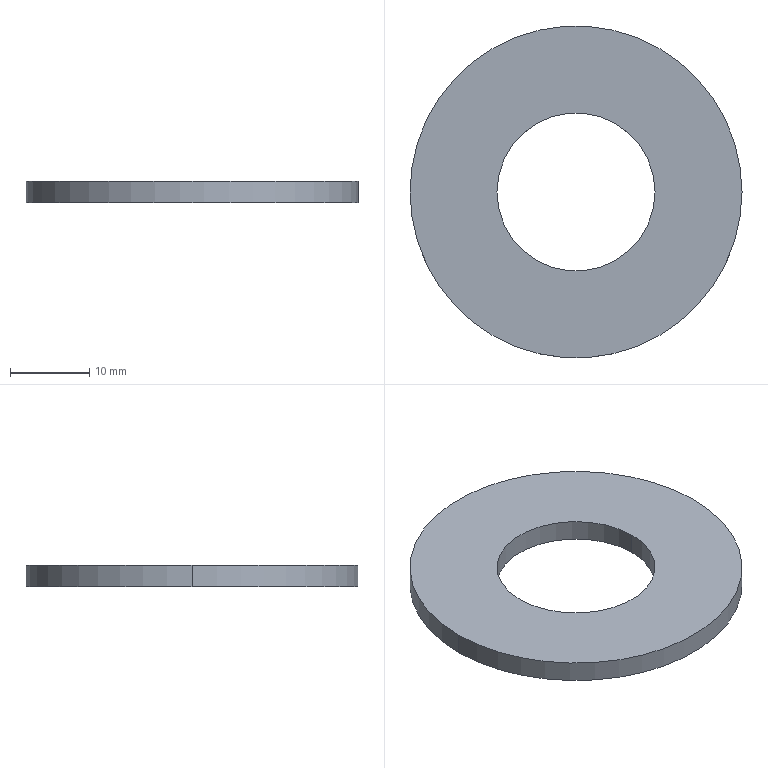Part | STEP file | Pin washer nut at M20 | 1 solid | 6 faces | box 42 x 42 x 2.7 mm | volume 2892 mm3 | cylinder 4 | plane 2 | commonest cylinder face diameters 20 x2 42 x2
STEP:
#1=CARTESIAN_POINT('',(-10.,0.,2.7));
#2=VERTEX_POINT('',#1);
#3=CARTESIAN_POINT('',(10.,0.,2.7));
#4=VERTEX_POINT('',#3);
#5=CARTESIAN_POINT('',(0.,0.,2.7));
#6=DIRECTION('',(0.,0.,1.));
#7=DIRECTION('',(1.,0.,0.));
#8=AXIS2_PLACEMENT_3D('',#5,#6,#7);
#9=CIRCLE('',#8,10.);
#10=EDGE_CURVE('',#2,#4,#9,.T.);
#11=ORIENTED_EDGE('',*,*,#10,.T.);
#12=CARTESIAN_POINT('',(10.,0.,0.));
#13=VERTEX_POINT('',#12);
#14=CARTESIAN_POINT('',(10.,0.,2.7));
#15=DIRECTION('',(0.,0.,-1.));
#16=VECTOR('',#15,1000.);
#17=LINE('',#14,#16);
#18=EDGE_CURVE('',#4,#13,#17,.T.);
#19=ORIENTED_EDGE('',*,*,#18,.T.);
#20=CARTESIAN_POINT('',(-10.,0.,0.));
#21=VERTEX_POINT('',#20);
#22=CARTESIAN_POINT('',(0.,0.,0.));
#23=DIRECTION('',(0.,0.,1.));
#24=DIRECTION('',(1.,0.,0.));
#25=AXIS2_PLACEMENT_3D('',#22,#23,#24);
#26=CIRCLE('',#25,10.);
#27=EDGE_CURVE('',#21,#13,#26,.T.);
#28=ORIENTED_EDGE('',*,*,#27,.F.);
#29=CARTESIAN_POINT('',(-10.,0.,2.7));
#30=DIRECTION('',(0.,0.,-1.));
#31=VECTOR('',#30,1000.);
#32=LINE('',#29,#31);
#33=EDGE_CURVE('',#2,#21,#32,.T.);
#34=ORIENTED_EDGE('',*,*,#33,.F.);
#35=EDGE_LOOP('',(#11,#19,#28,#34));
#36=FACE_OUTER_BOUND('',#35,.T.);
#37=CARTESIAN_POINT('',(0.,0.,2.7));
#38=DIRECTION('',(0.,0.,-1.));
#39=DIRECTION('',(-1.,0.,0.));
#40=AXIS2_PLACEMENT_3D('',#37,#38,#39);
#41=CYLINDRICAL_SURFACE('',#40,10.);
#42=ADVANCED_FACE('',(#36),#41,.F.);
#43=CARTESIAN_POINT('',(21.,0.,2.7));
#44=VERTEX_POINT('',#43);
#45=CARTESIAN_POINT('',(-21.,0.,2.7));
#46=VERTEX_POINT('',#45);
#47=CARTESIAN_POINT('',(0.,0.,2.7));
#48=DIRECTION('',(0.,0.,1.));
#49=DIRECTION('',(1.,0.,0.));
#50=AXIS2_PLACEMENT_3D('',#47,#48,#49);
#51=CIRCLE('',#50,21.);
#52=EDGE_CURVE('',#44,#46,#51,.T.);
#53=ORIENTED_EDGE('',*,*,#52,.F.);
#54=CARTESIAN_POINT('',(21.,0.,0.));
#55=VERTEX_POINT('',#54);
#56=CARTESIAN_POINT('',(21.,0.,2.7));
#57=DIRECTION('',(0.,0.,-1.));
#58=VECTOR('',#57,1000.);
#59=LINE('',#56,#58);
#60=EDGE_CURVE('',#44,#55,#59,.T.);
#61=ORIENTED_EDGE('',*,*,#60,.T.);
#62=CARTESIAN_POINT('',(-21.,0.,0.));
#63=VERTEX_POINT('',#62);
#64=CARTESIAN_POINT('',(0.,0.,0.));
#65=DIRECTION('',(0.,0.,1.));
#66=DIRECTION('',(1.,0.,0.));
#67=AXIS2_PLACEMENT_3D('',#64,#65,#66);
#68=CIRCLE('',#67,21.);
#69=EDGE_CURVE('',#55,#63,#68,.T.);
#70=ORIENTED_EDGE('',*,*,#69,.T.);
#71=CARTESIAN_POINT('',(-21.,0.,2.7));
#72=DIRECTION('',(0.,0.,-1.));
#73=VECTOR('',#72,1000.);
#74=LINE('',#71,#73);
#75=EDGE_CURVE('',#46,#63,#74,.T.);
#76=ORIENTED_EDGE('',*,*,#75,.F.);
#77=EDGE_LOOP('',(#53,#61,#70,#76));
#78=FACE_OUTER_BOUND('',#77,.T.);
#79=CARTESIAN_POINT('',(0.,0.,2.7));
#80=DIRECTION('',(0.,0.,-1.));
#81=DIRECTION('',(-1.,0.,0.));
#82=AXIS2_PLACEMENT_3D('',#79,#80,#81);
#83=CYLINDRICAL_SURFACE('',#82,21.);
#84=ADVANCED_FACE('',(#78),#83,.T.);
#85=CARTESIAN_POINT('',(0.,0.,2.7));
#86=DIRECTION('',(0.,0.,1.));
#87=DIRECTION('',(1.,0.,0.));
#88=AXIS2_PLACEMENT_3D('',#85,#86,#87);
#89=CIRCLE('',#88,21.);
#90=EDGE_CURVE('',#46,#44,#89,.T.);
#91=ORIENTED_EDGE('',*,*,#90,.T.);
#92=ORIENTED_EDGE('',*,*,#52,.T.);
#93=EDGE_LOOP('',(#91,#92));
#94=FACE_OUTER_BOUND('',#93,.T.);
#95=ORIENTED_EDGE('',*,*,#10,.F.);
#96=CARTESIAN_POINT('',(0.,0.,2.7));
#97=DIRECTION('',(0.,0.,1.));
#98=DIRECTION('',(1.,0.,0.));
#99=AXIS2_PLACEMENT_3D('',#96,#97,#98);
#100=CIRCLE('',#99,10.);
#101=EDGE_CURVE('',#4,#2,#100,.T.);
#102=ORIENTED_EDGE('',*,*,#101,.F.);
#103=EDGE_LOOP('',(#95,#102));
#104=FACE_BOUND('',#103,.T.);
#105=CARTESIAN_POINT('',(0.,0.,2.7));
#106=DIRECTION('',(0.,0.,1.));
#107=DIRECTION('',(1.,0.,0.));
#108=AXIS2_PLACEMENT_3D('',#105,#106,#107);
#109=PLANE('',#108);
#110=ADVANCED_FACE('',(#94,#104),#109,.T.);
#111=CARTESIAN_POINT('',(0.,0.,0.));
#112=DIRECTION('',(0.,0.,1.));
#113=DIRECTION('',(1.,0.,0.));
#114=AXIS2_PLACEMENT_3D('',#111,#112,#113);
#115=CIRCLE('',#114,21.);
#116=EDGE_CURVE('',#63,#55,#115,.T.);
#117=ORIENTED_EDGE('',*,*,#116,.F.);
#118=ORIENTED_EDGE('',*,*,#69,.F.);
#119=EDGE_LOOP('',(#117,#118));
#120=FACE_OUTER_BOUND('',#119,.T.);
#121=ORIENTED_EDGE('',*,*,#27,.T.);
#122=CARTESIAN_POINT('',(0.,0.,0.));
#123=DIRECTION('',(0.,0.,1.));
#124=DIRECTION('',(1.,0.,0.));
#125=AXIS2_PLACEMENT_3D('',#122,#123,#124);
#126=CIRCLE('',#125,10.);
#127=EDGE_CURVE('',#13,#21,#126,.T.);
#128=ORIENTED_EDGE('',*,*,#127,.T.);
#129=EDGE_LOOP('',(#121,#128));
#130=FACE_BOUND('',#129,.T.);
#131=CARTESIAN_POINT('',(0.,0.,0.));
#132=DIRECTION('',(0.,0.,1.));
#133=DIRECTION('',(1.,0.,0.));
#134=AXIS2_PLACEMENT_3D('',#131,#132,#133);
#135=PLANE('',#134);
#136=ADVANCED_FACE('',(#120,#130),#135,.F.);
#137=ORIENTED_EDGE('',*,*,#60,.F.);
#138=ORIENTED_EDGE('',*,*,#90,.F.);
#139=ORIENTED_EDGE('',*,*,#75,.T.);
#140=ORIENTED_EDGE('',*,*,#116,.T.);
#141=EDGE_LOOP('',(#137,#138,#139,#140));
#142=FACE_OUTER_BOUND('',#141,.T.);
#143=CARTESIAN_POINT('',(0.,0.,2.7));
#144=DIRECTION('',(0.,0.,-1.));
#145=DIRECTION('',(-1.,0.,0.));
#146=AXIS2_PLACEMENT_3D('',#143,#144,#145);
#147=CYLINDRICAL_SURFACE('',#146,21.);
#148=ADVANCED_FACE('',(#142),#147,.T.);
#149=ORIENTED_EDGE('',*,*,#18,.F.);
#150=ORIENTED_EDGE('',*,*,#101,.T.);
#151=ORIENTED_EDGE('',*,*,#33,.T.);
#152=ORIENTED_EDGE('',*,*,#127,.F.);
#153=EDGE_LOOP('',(#149,#150,#151,#152));
#154=FACE_OUTER_BOUND('',#153,.T.);
#155=CARTESIAN_POINT('',(0.,0.,2.7));
#156=DIRECTION('',(0.,0.,-1.));
#157=DIRECTION('',(-1.,0.,0.));
#158=AXIS2_PLACEMENT_3D('',#155,#156,#157);
#159=CYLINDRICAL_SURFACE('',#158,10.);
#160=ADVANCED_FACE('',(#154),#159,.F.);
#161=CLOSED_SHELL('',(#42,#84,#110,#136,#148,#160));
#162=MANIFOLD_SOLID_BREP('',#161);
#163=CARTESIAN_POINT('',(0.,0.,0.));
#164=DIRECTION('',(0.,0.,1.));
#165=DIRECTION('',(1.,0.,0.));
#166=AXIS2_PLACEMENT_3D('',#163,#164,#165);
#167=(LENGTH_UNIT()NAMED_UNIT(*)SI_UNIT(.MILLI.,.METRE.));
#168=UNCERTAINTY_MEASURE_WITH_UNIT(LENGTH_MEASURE(0.00001),#167,'','');
#169=(NAMED_UNIT(*)PLANE_ANGLE_UNIT()SI_UNIT($,.RADIAN.));
#170=(NAMED_UNIT(*)SI_UNIT($,.STERADIAN.)SOLID_ANGLE_UNIT());
#171=(GEOMETRIC_REPRESENTATION_CONTEXT(3)GLOBAL_UNCERTAINTY_ASSIGNED_CONTEXT((#168))GLOBAL_UNIT_ASSIGNED_CONTEXT((#167,#169,#170))REPRESENTATION_CONTEXT('',''));
#172=ADVANCED_BREP_SHAPE_REPRESENTATION('',(#162,#166),#171);